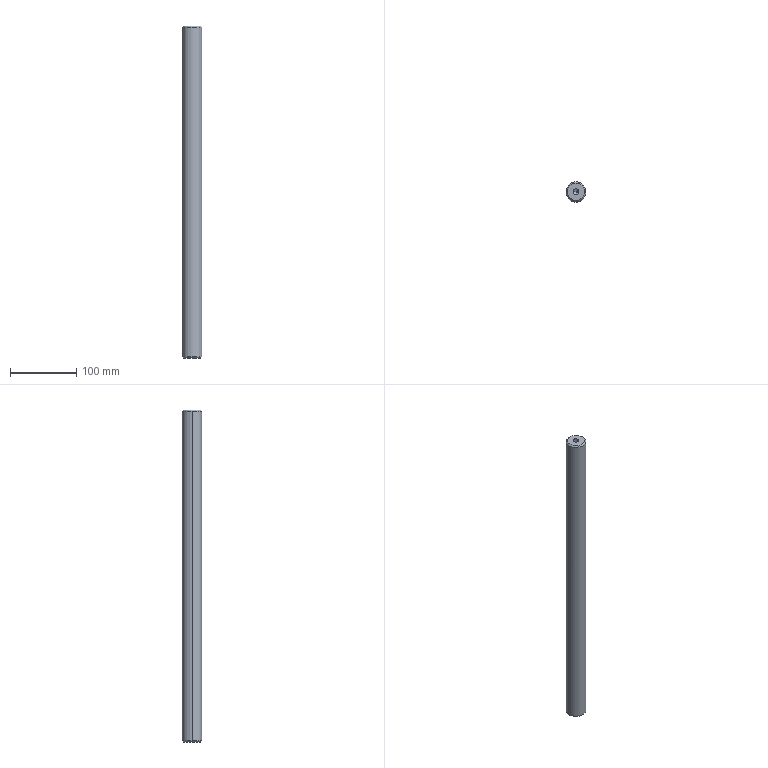Part | SolidWorks | features Chamfer 1, Extrusion 1, HoleWzd 1 | 1 solid | 12 faces | box 30 x 30 x 500 mm | volume 351630 mm3 | cone 6 | cylinder 4 | plane 2 | commonest cylinder face diameters 8.5 x2 30 x2
STEP:
#1=CARTESIAN_POINT('',(-4.25,0.,475.5));
#2=VERTEX_POINT('',#1);
#3=CARTESIAN_POINT('',(4.25,0.,475.5));
#4=VERTEX_POINT('',#3);
#5=CARTESIAN_POINT('',(0.,0.,475.5));
#6=DIRECTION('',(0.,0.,1.));
#7=DIRECTION('',(1.,0.,0.));
#8=AXIS2_PLACEMENT_3D('',#5,#6,#7);
#9=CIRCLE('',#8,4.25);
#10=EDGE_CURVE('',#2,#4,#9,.T.);
#11=ORIENTED_EDGE('',*,*,#10,.F.);
#12=CARTESIAN_POINT('',(-4.25,0.,500.));
#13=VERTEX_POINT('',#12);
#14=CARTESIAN_POINT('',(-4.25,0.,500.));
#15=DIRECTION('',(0.,0.,1.));
#16=VECTOR('',#15,1000.);
#17=LINE('',#14,#16);
#18=EDGE_CURVE('',#2,#13,#17,.T.);
#19=ORIENTED_EDGE('',*,*,#18,.T.);
#20=CARTESIAN_POINT('',(4.25,0.,500.));
#21=VERTEX_POINT('',#20);
#22=CARTESIAN_POINT('',(0.,0.,500.));
#23=DIRECTION('',(0.,0.,1.));
#24=DIRECTION('',(1.,0.,0.));
#25=AXIS2_PLACEMENT_3D('',#22,#23,#24);
#26=CIRCLE('',#25,4.25);
#27=EDGE_CURVE('',#13,#21,#26,.T.);
#28=ORIENTED_EDGE('',*,*,#27,.T.);
#29=CARTESIAN_POINT('',(4.25,0.,500.));
#30=DIRECTION('',(0.,0.,1.));
#31=VECTOR('',#30,1000.);
#32=LINE('',#29,#31);
#33=EDGE_CURVE('',#4,#21,#32,.T.);
#34=ORIENTED_EDGE('',*,*,#33,.F.);
#35=EDGE_LOOP('',(#11,#19,#28,#34));
#36=FACE_OUTER_BOUND('',#35,.T.);
#37=CARTESIAN_POINT('',(0.,0.,500.));
#38=DIRECTION('',(0.,0.,1.));
#39=DIRECTION('',(1.,0.,0.));
#40=AXIS2_PLACEMENT_3D('',#37,#38,#39);
#41=CYLINDRICAL_SURFACE('',#40,4.25);
#42=ADVANCED_FACE('',(#36),#41,.F.);
#43=CARTESIAN_POINT('',(0.,0.,472.946));
#44=VERTEX_POINT('',#43);
#45=CARTESIAN_POINT('',(4.25,0.,475.5));
#46=DIRECTION('',(0.8572,0.,0.515));
#47=VECTOR('',#46,1000.);
#48=LINE('',#45,#47);
#49=EDGE_CURVE('',#44,#4,#48,.T.);
#50=ORIENTED_EDGE('',*,*,#49,.F.);
#51=CARTESIAN_POINT('',(-4.25,0.,475.5));
#52=DIRECTION('',(-0.8572,0.,0.515));
#53=VECTOR('',#52,1000.);
#54=LINE('',#51,#53);
#55=EDGE_CURVE('',#44,#2,#54,.T.);
#56=ORIENTED_EDGE('',*,*,#55,.T.);
#57=ORIENTED_EDGE('',*,*,#10,.T.);
#58=EDGE_LOOP('',(#50,#56,#57));
#59=FACE_OUTER_BOUND('',#58,.T.);
#60=CARTESIAN_POINT('',(0.,0.,475.5));
#61=DIRECTION('',(0.,0.,1.));
#62=DIRECTION('',(1.,0.,0.));
#63=AXIS2_PLACEMENT_3D('',#60,#61,#62);
#64=CONICAL_SURFACE('',#63,4.25,1.03);
#65=ADVANCED_FACE('',(#59),#64,.F.);
#66=CARTESIAN_POINT('',(-13.,0.,0.));
#67=VERTEX_POINT('',#66);
#68=CARTESIAN_POINT('',(13.,0.,0.));
#69=VERTEX_POINT('',#68);
#70=CARTESIAN_POINT('',(0.,0.,0.));
#71=DIRECTION('',(0.,0.,-1.));
#72=DIRECTION('',(1.,0.,0.));
#73=AXIS2_PLACEMENT_3D('',#70,#71,#72);
#74=CIRCLE('',#73,13.);
#75=EDGE_CURVE('',#67,#69,#74,.T.);
#76=ORIENTED_EDGE('',*,*,#75,.F.);
#77=CARTESIAN_POINT('',(-15.,0.,2.));
#78=VERTEX_POINT('',#77);
#79=CARTESIAN_POINT('',(-15.,0.,2.));
#80=DIRECTION('',(-0.7071,0.,0.7071));
#81=VECTOR('',#80,1000.);
#82=LINE('',#79,#81);
#83=EDGE_CURVE('',#67,#78,#82,.T.);
#84=ORIENTED_EDGE('',*,*,#83,.T.);
#85=CARTESIAN_POINT('',(15.,0.,2.));
#86=VERTEX_POINT('',#85);
#87=CARTESIAN_POINT('',(0.,0.,2.));
#88=DIRECTION('',(0.,0.,1.));
#89=DIRECTION('',(1.,0.,0.));
#90=AXIS2_PLACEMENT_3D('',#87,#88,#89);
#91=CIRCLE('',#90,15.);
#92=EDGE_CURVE('',#86,#78,#91,.T.);
#93=ORIENTED_EDGE('',*,*,#92,.F.);
#94=CARTESIAN_POINT('',(15.,0.,2.));
#95=DIRECTION('',(0.7071,0.,0.7071));
#96=VECTOR('',#95,1000.);
#97=LINE('',#94,#96);
#98=EDGE_CURVE('',#69,#86,#97,.T.);
#99=ORIENTED_EDGE('',*,*,#98,.F.);
#100=EDGE_LOOP('',(#76,#84,#93,#99));
#101=FACE_OUTER_BOUND('',#100,.T.);
#102=CARTESIAN_POINT('',(0.,0.,2.));
#103=DIRECTION('',(0.,0.,1.));
#104=DIRECTION('',(1.,0.,0.));
#105=AXIS2_PLACEMENT_3D('',#102,#103,#104);
#106=CONICAL_SURFACE('',#105,15.,0.7854);
#107=ADVANCED_FACE('',(#101),#106,.T.);
#108=CARTESIAN_POINT('',(13.,0.,500.));
#109=VERTEX_POINT('',#108);
#110=CARTESIAN_POINT('',(-13.,0.,500.));
#111=VERTEX_POINT('',#110);
#112=CARTESIAN_POINT('',(0.,0.,500.));
#113=DIRECTION('',(0.,0.,1.));
#114=DIRECTION('',(1.,0.,0.));
#115=AXIS2_PLACEMENT_3D('',#112,#113,#114);
#116=CIRCLE('',#115,13.);
#117=EDGE_CURVE('',#109,#111,#116,.T.);
#118=ORIENTED_EDGE('',*,*,#117,.F.);
#119=CARTESIAN_POINT('',(15.,0.,498.));
#120=VERTEX_POINT('',#119);
#121=CARTESIAN_POINT('',(13.,0.,500.));
#122=DIRECTION('',(0.7071,0.,-0.7071));
#123=VECTOR('',#122,1000.);
#124=LINE('',#121,#123);
#125=EDGE_CURVE('',#109,#120,#124,.T.);
#126=ORIENTED_EDGE('',*,*,#125,.T.);
#127=CARTESIAN_POINT('',(-15.,0.,498.));
#128=VERTEX_POINT('',#127);
#129=CARTESIAN_POINT('',(0.,0.,498.));
#130=DIRECTION('',(0.,0.,-1.));
#131=DIRECTION('',(1.,0.,0.));
#132=AXIS2_PLACEMENT_3D('',#129,#130,#131);
#133=CIRCLE('',#132,15.);
#134=EDGE_CURVE('',#128,#120,#133,.T.);
#135=ORIENTED_EDGE('',*,*,#134,.F.);
#136=CARTESIAN_POINT('',(-13.,0.,500.));
#137=DIRECTION('',(-0.7071,0.,-0.7071));
#138=VECTOR('',#137,1000.);
#139=LINE('',#136,#138);
#140=EDGE_CURVE('',#111,#128,#139,.T.);
#141=ORIENTED_EDGE('',*,*,#140,.F.);
#142=EDGE_LOOP('',(#118,#126,#135,#141));
#143=FACE_OUTER_BOUND('',#142,.T.);
#144=CARTESIAN_POINT('',(0.,0.,500.));
#145=DIRECTION('',(0.,0.,-1.));
#146=DIRECTION('',(-1.,0.,0.));
#147=AXIS2_PLACEMENT_3D('',#144,#145,#146);
#148=CONICAL_SURFACE('',#147,13.,0.7854);
#149=ADVANCED_FACE('',(#143),#148,.T.);
#150=ORIENTED_EDGE('',*,*,#134,.T.);
#151=CARTESIAN_POINT('',(15.,0.,500.));
#152=DIRECTION('',(0.,0.,-1.));
#153=VECTOR('',#152,1000.);
#154=LINE('',#151,#153);
#155=EDGE_CURVE('',#120,#86,#154,.T.);
#156=ORIENTED_EDGE('',*,*,#155,.T.);
#157=ORIENTED_EDGE('',*,*,#92,.T.);
#158=CARTESIAN_POINT('',(-15.,0.,500.));
#159=DIRECTION('',(0.,0.,-1.));
#160=VECTOR('',#159,1000.);
#161=LINE('',#158,#160);
#162=EDGE_CURVE('',#128,#78,#161,.T.);
#163=ORIENTED_EDGE('',*,*,#162,.F.);
#164=EDGE_LOOP('',(#150,#156,#157,#163));
#165=FACE_OUTER_BOUND('',#164,.T.);
#166=CARTESIAN_POINT('',(0.,0.,500.));
#167=DIRECTION('',(0.,0.,-1.));
#168=DIRECTION('',(-1.,0.,0.));
#169=AXIS2_PLACEMENT_3D('',#166,#167,#168);
#170=CYLINDRICAL_SURFACE('',#169,15.);
#171=ADVANCED_FACE('',(#165),#170,.T.);
#172=ORIENTED_EDGE('',*,*,#155,.F.);
#173=CARTESIAN_POINT('',(0.,0.,498.));
#174=DIRECTION('',(0.,0.,-1.));
#175=DIRECTION('',(1.,0.,0.));
#176=AXIS2_PLACEMENT_3D('',#173,#174,#175);
#177=CIRCLE('',#176,15.);
#178=EDGE_CURVE('',#120,#128,#177,.T.);
#179=ORIENTED_EDGE('',*,*,#178,.T.);
#180=ORIENTED_EDGE('',*,*,#162,.T.);
#181=CARTESIAN_POINT('',(0.,0.,2.));
#182=DIRECTION('',(0.,0.,1.));
#183=DIRECTION('',(1.,0.,0.));
#184=AXIS2_PLACEMENT_3D('',#181,#182,#183);
#185=CIRCLE('',#184,15.);
#186=EDGE_CURVE('',#78,#86,#185,.T.);
#187=ORIENTED_EDGE('',*,*,#186,.T.);
#188=EDGE_LOOP('',(#172,#179,#180,#187));
#189=FACE_OUTER_BOUND('',#188,.T.);
#190=CARTESIAN_POINT('',(0.,0.,500.));
#191=DIRECTION('',(0.,0.,-1.));
#192=DIRECTION('',(-1.,0.,0.));
#193=AXIS2_PLACEMENT_3D('',#190,#191,#192);
#194=CYLINDRICAL_SURFACE('',#193,15.);
#195=ADVANCED_FACE('',(#189),#194,.T.);
#196=CARTESIAN_POINT('',(0.,0.,500.));
#197=DIRECTION('',(0.,0.,1.));
#198=DIRECTION('',(1.,0.,0.));
#199=AXIS2_PLACEMENT_3D('',#196,#197,#198);
#200=CIRCLE('',#199,4.25);
#201=EDGE_CURVE('',#21,#13,#200,.T.);
#202=ORIENTED_EDGE('',*,*,#201,.F.);
#203=ORIENTED_EDGE('',*,*,#27,.F.);
#204=EDGE_LOOP('',(#202,#203));
#205=FACE_BOUND('',#204,.T.);
#206=CARTESIAN_POINT('',(0.,0.,500.));
#207=DIRECTION('',(0.,0.,1.));
#208=DIRECTION('',(1.,0.,0.));
#209=AXIS2_PLACEMENT_3D('',#206,#207,#208);
#210=CIRCLE('',#209,13.);
#211=EDGE_CURVE('',#111,#109,#210,.T.);
#212=ORIENTED_EDGE('',*,*,#211,.T.);
#213=ORIENTED_EDGE('',*,*,#117,.T.);
#214=EDGE_LOOP('',(#212,#213));
#215=FACE_OUTER_BOUND('',#214,.T.);
#216=CARTESIAN_POINT('',(0.,0.,500.));
#217=DIRECTION('',(0.,0.,1.));
#218=DIRECTION('',(1.,0.,0.));
#219=AXIS2_PLACEMENT_3D('',#216,#217,#218);
#220=PLANE('',#219);
#221=ADVANCED_FACE('',(#205,#215),#220,.T.);
#222=CARTESIAN_POINT('',(0.,0.,0.));
#223=DIRECTION('',(0.,0.,-1.));
#224=DIRECTION('',(1.,0.,0.));
#225=AXIS2_PLACEMENT_3D('',#222,#223,#224);
#226=CIRCLE('',#225,13.);
#227=EDGE_CURVE('',#69,#67,#226,.T.);
#228=ORIENTED_EDGE('',*,*,#227,.T.);
#229=ORIENTED_EDGE('',*,*,#75,.T.);
#230=EDGE_LOOP('',(#228,#229));
#231=FACE_OUTER_BOUND('',#230,.T.);
#232=CARTESIAN_POINT('',(0.,0.,0.));
#233=DIRECTION('',(0.,0.,1.));
#234=DIRECTION('',(1.,0.,0.));
#235=AXIS2_PLACEMENT_3D('',#232,#233,#234);
#236=PLANE('',#235);
#237=ADVANCED_FACE('',(#231),#236,.F.);
#238=ORIENTED_EDGE('',*,*,#125,.F.);
#239=ORIENTED_EDGE('',*,*,#211,.F.);
#240=ORIENTED_EDGE('',*,*,#140,.T.);
#241=ORIENTED_EDGE('',*,*,#178,.F.);
#242=EDGE_LOOP('',(#238,#239,#240,#241));
#243=FACE_OUTER_BOUND('',#242,.T.);
#244=CARTESIAN_POINT('',(0.,0.,500.));
#245=DIRECTION('',(0.,0.,-1.));
#246=DIRECTION('',(-1.,0.,0.));
#247=AXIS2_PLACEMENT_3D('',#244,#245,#246);
#248=CONICAL_SURFACE('',#247,13.,0.7854);
#249=ADVANCED_FACE('',(#243),#248,.T.);
#250=ORIENTED_EDGE('',*,*,#83,.F.);
#251=ORIENTED_EDGE('',*,*,#227,.F.);
#252=ORIENTED_EDGE('',*,*,#98,.T.);
#253=ORIENTED_EDGE('',*,*,#186,.F.);
#254=EDGE_LOOP('',(#250,#251,#252,#253));
#255=FACE_OUTER_BOUND('',#254,.T.);
#256=CARTESIAN_POINT('',(0.,0.,2.));
#257=DIRECTION('',(0.,0.,1.));
#258=DIRECTION('',(1.,0.,0.));
#259=AXIS2_PLACEMENT_3D('',#256,#257,#258);
#260=CONICAL_SURFACE('',#259,15.,0.7854);
#261=ADVANCED_FACE('',(#255),#260,.T.);
#262=ORIENTED_EDGE('',*,*,#55,.F.);
#263=ORIENTED_EDGE('',*,*,#49,.T.);
#264=CARTESIAN_POINT('',(0.,0.,475.5));
#265=DIRECTION('',(0.,0.,1.));
#266=DIRECTION('',(1.,0.,0.));
#267=AXIS2_PLACEMENT_3D('',#264,#265,#266);
#268=CIRCLE('',#267,4.25);
#269=EDGE_CURVE('',#4,#2,#268,.T.);
#270=ORIENTED_EDGE('',*,*,#269,.T.);
#271=EDGE_LOOP('',(#262,#263,#270));
#272=FACE_OUTER_BOUND('',#271,.T.);
#273=CARTESIAN_POINT('',(0.,0.,475.5));
#274=DIRECTION('',(0.,0.,1.));
#275=DIRECTION('',(1.,0.,0.));
#276=AXIS2_PLACEMENT_3D('',#273,#274,#275);
#277=CONICAL_SURFACE('',#276,4.25,1.03);
#278=ADVANCED_FACE('',(#272),#277,.F.);
#279=ORIENTED_EDGE('',*,*,#18,.F.);
#280=ORIENTED_EDGE('',*,*,#269,.F.);
#281=ORIENTED_EDGE('',*,*,#33,.T.);
#282=ORIENTED_EDGE('',*,*,#201,.T.);
#283=EDGE_LOOP('',(#279,#280,#281,#282));
#284=FACE_OUTER_BOUND('',#283,.T.);
#285=CARTESIAN_POINT('',(0.,0.,500.));
#286=DIRECTION('',(0.,0.,1.));
#287=DIRECTION('',(1.,0.,0.));
#288=AXIS2_PLACEMENT_3D('',#285,#286,#287);
#289=CYLINDRICAL_SURFACE('',#288,4.25);
#290=ADVANCED_FACE('',(#284),#289,.F.);
#291=CLOSED_SHELL('',(#42,#65,#107,#149,#171,#195,#221,#237,#249,#261,#278,#290));
#292=MANIFOLD_SOLID_BREP('',#291);
#293=CARTESIAN_POINT('',(0.,0.,0.));
#294=DIRECTION('',(0.,0.,1.));
#295=DIRECTION('',(1.,0.,0.));
#296=AXIS2_PLACEMENT_3D('',#293,#294,#295);
#297=(LENGTH_UNIT()NAMED_UNIT(*)SI_UNIT(.MILLI.,.METRE.));
#298=UNCERTAINTY_MEASURE_WITH_UNIT(LENGTH_MEASURE(0.00001),#297,'','');
#299=(NAMED_UNIT(*)PLANE_ANGLE_UNIT()SI_UNIT($,.RADIAN.));
#300=(NAMED_UNIT(*)SI_UNIT($,.STERADIAN.)SOLID_ANGLE_UNIT());
#301=(GEOMETRIC_REPRESENTATION_CONTEXT(3)GLOBAL_UNCERTAINTY_ASSIGNED_CONTEXT((#298))GLOBAL_UNIT_ASSIGNED_CONTEXT((#297,#299,#300))REPRESENTATION_CONTEXT('',''));
#302=ADVANCED_BREP_SHAPE_REPRESENTATION('',(#292,#296),#301);